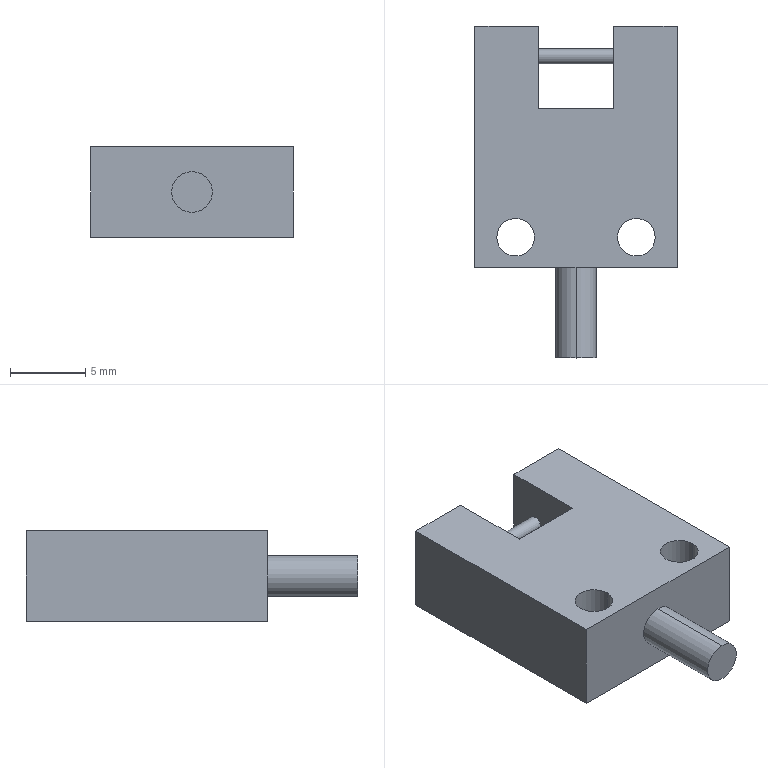Part | SolidWorks | features ICE 3, Extrusion 1, HoleWzd 1 | 1 solid | 19 faces | box 13.4 x 22 x 6 mm | volume 1101 mm3 | plane 11 | cylinder 8 | commonest cylinder face diameters 2.5 x4 1 x2 2.7 x2
STEP:
#1=CARTESIAN_POINT('',(-2.5,6.5,0.));
#2=VERTEX_POINT('',#1);
#3=CARTESIAN_POINT('',(-2.5,5.5,0.));
#4=VERTEX_POINT('',#3);
#5=CARTESIAN_POINT('',(-2.5,6.,0.));
#6=DIRECTION('',(1.,0.,0.));
#7=DIRECTION('',(0.,-1.,0.));
#8=AXIS2_PLACEMENT_3D('',#5,#6,#7);
#9=CIRCLE('',#8,0.5);
#10=EDGE_CURVE('',#2,#4,#9,.T.);
#11=ORIENTED_EDGE('',*,*,#10,.T.);
#12=CARTESIAN_POINT('',(2.5,5.5,0.));
#13=VERTEX_POINT('',#12);
#14=CARTESIAN_POINT('',(-3.914,5.5,0.));
#15=DIRECTION('',(1.,0.,0.));
#16=VECTOR('',#15,1000.);
#17=LINE('',#14,#16);
#18=EDGE_CURVE('',#4,#13,#17,.T.);
#19=ORIENTED_EDGE('',*,*,#18,.T.);
#20=CARTESIAN_POINT('',(2.5,6.5,0.));
#21=VERTEX_POINT('',#20);
#22=CARTESIAN_POINT('',(2.5,6.,0.));
#23=DIRECTION('',(-1.,0.,0.));
#24=DIRECTION('',(0.,1.,0.));
#25=AXIS2_PLACEMENT_3D('',#22,#23,#24);
#26=CIRCLE('',#25,0.5);
#27=EDGE_CURVE('',#13,#21,#26,.T.);
#28=ORIENTED_EDGE('',*,*,#27,.T.);
#29=CARTESIAN_POINT('',(-3.914,6.5,0.));
#30=DIRECTION('',(1.,0.,0.));
#31=VECTOR('',#30,1000.);
#32=LINE('',#29,#31);
#33=EDGE_CURVE('',#2,#21,#32,.T.);
#34=ORIENTED_EDGE('',*,*,#33,.F.);
#35=EDGE_LOOP('',(#11,#19,#28,#34));
#36=FACE_OUTER_BOUND('',#35,.T.);
#37=CARTESIAN_POINT('',(-3.914,6.,0.));
#38=DIRECTION('',(1.,0.,0.));
#39=DIRECTION('',(0.,1.,0.));
#40=AXIS2_PLACEMENT_3D('',#37,#38,#39);
#41=CYLINDRICAL_SURFACE('',#40,0.5);
#42=ADVANCED_FACE('',(#36),#41,.T.);
#43=CARTESIAN_POINT('',(-5.25,-6.,-3.));
#44=VERTEX_POINT('',#43);
#45=CARTESIAN_POINT('',(-2.75,-6.,-3.));
#46=VERTEX_POINT('',#45);
#47=CARTESIAN_POINT('',(-4.,-6.,-3.));
#48=DIRECTION('',(0.,0.,1.));
#49=DIRECTION('',(1.,0.,0.));
#50=AXIS2_PLACEMENT_3D('',#47,#48,#49);
#51=CIRCLE('',#50,1.25);
#52=EDGE_CURVE('',#44,#46,#51,.T.);
#53=ORIENTED_EDGE('',*,*,#52,.F.);
#54=CARTESIAN_POINT('',(-5.25,-6.,3.));
#55=VERTEX_POINT('',#54);
#56=CARTESIAN_POINT('',(-5.25,-6.,3.));
#57=DIRECTION('',(0.,0.,1.));
#58=VECTOR('',#57,1000.);
#59=LINE('',#56,#58);
#60=EDGE_CURVE('',#44,#55,#59,.T.);
#61=ORIENTED_EDGE('',*,*,#60,.T.);
#62=CARTESIAN_POINT('',(-2.75,-6.,3.));
#63=VERTEX_POINT('',#62);
#64=CARTESIAN_POINT('',(-4.,-6.,3.));
#65=DIRECTION('',(0.,0.,1.));
#66=DIRECTION('',(1.,0.,0.));
#67=AXIS2_PLACEMENT_3D('',#64,#65,#66);
#68=CIRCLE('',#67,1.25);
#69=EDGE_CURVE('',#55,#63,#68,.T.);
#70=ORIENTED_EDGE('',*,*,#69,.T.);
#71=CARTESIAN_POINT('',(-2.75,-6.,3.));
#72=DIRECTION('',(0.,0.,1.));
#73=VECTOR('',#72,1000.);
#74=LINE('',#71,#73);
#75=EDGE_CURVE('',#46,#63,#74,.T.);
#76=ORIENTED_EDGE('',*,*,#75,.F.);
#77=EDGE_LOOP('',(#53,#61,#70,#76));
#78=FACE_OUTER_BOUND('',#77,.T.);
#79=CARTESIAN_POINT('',(-4.,-6.,3.));
#80=DIRECTION('',(0.,0.,1.));
#81=DIRECTION('',(1.,0.,0.));
#82=AXIS2_PLACEMENT_3D('',#79,#80,#81);
#83=CYLINDRICAL_SURFACE('',#82,1.25);
#84=ADVANCED_FACE('',(#78),#83,.F.);
#85=CARTESIAN_POINT('',(2.75,-6.,-3.));
#86=VERTEX_POINT('',#85);
#87=CARTESIAN_POINT('',(5.25,-6.,-3.));
#88=VERTEX_POINT('',#87);
#89=CARTESIAN_POINT('',(4.,-6.,-3.));
#90=DIRECTION('',(0.,0.,1.));
#91=DIRECTION('',(1.,0.,0.));
#92=AXIS2_PLACEMENT_3D('',#89,#90,#91);
#93=CIRCLE('',#92,1.25);
#94=EDGE_CURVE('',#86,#88,#93,.T.);
#95=ORIENTED_EDGE('',*,*,#94,.F.);
#96=CARTESIAN_POINT('',(2.75,-6.,3.));
#97=VERTEX_POINT('',#96);
#98=CARTESIAN_POINT('',(2.75,-6.,3.));
#99=DIRECTION('',(0.,0.,1.));
#100=VECTOR('',#99,1000.);
#101=LINE('',#98,#100);
#102=EDGE_CURVE('',#86,#97,#101,.T.);
#103=ORIENTED_EDGE('',*,*,#102,.T.);
#104=CARTESIAN_POINT('',(5.25,-6.,3.));
#105=VERTEX_POINT('',#104);
#106=CARTESIAN_POINT('',(4.,-6.,3.));
#107=DIRECTION('',(0.,0.,1.));
#108=DIRECTION('',(1.,0.,0.));
#109=AXIS2_PLACEMENT_3D('',#106,#107,#108);
#110=CIRCLE('',#109,1.25);
#111=EDGE_CURVE('',#97,#105,#110,.T.);
#112=ORIENTED_EDGE('',*,*,#111,.T.);
#113=CARTESIAN_POINT('',(5.25,-6.,3.));
#114=DIRECTION('',(0.,0.,1.));
#115=VECTOR('',#114,1000.);
#116=LINE('',#113,#115);
#117=EDGE_CURVE('',#88,#105,#116,.T.);
#118=ORIENTED_EDGE('',*,*,#117,.F.);
#119=EDGE_LOOP('',(#95,#103,#112,#118));
#120=FACE_OUTER_BOUND('',#119,.T.);
#121=CARTESIAN_POINT('',(4.,-6.,3.));
#122=DIRECTION('',(0.,0.,1.));
#123=DIRECTION('',(1.,0.,0.));
#124=AXIS2_PLACEMENT_3D('',#121,#122,#123);
#125=CYLINDRICAL_SURFACE('',#124,1.25);
#126=ADVANCED_FACE('',(#120),#125,.F.);
#127=CARTESIAN_POINT('',(0.,-14.,-1.35));
#128=VERTEX_POINT('',#127);
#129=CARTESIAN_POINT('',(0.,-14.,1.35));
#130=VERTEX_POINT('',#129);
#131=CARTESIAN_POINT('',(0.,-14.,0.));
#132=DIRECTION('',(0.,-1.,0.));
#133=DIRECTION('',(0.,0.,-1.));
#134=AXIS2_PLACEMENT_3D('',#131,#132,#133);
#135=CIRCLE('',#134,1.35);
#136=EDGE_CURVE('',#128,#130,#135,.T.);
#137=ORIENTED_EDGE('',*,*,#136,.F.);
#138=CARTESIAN_POINT('',(0.,-8.,-1.35));
#139=VERTEX_POINT('',#138);
#140=CARTESIAN_POINT('',(0.,-14.,-1.35));
#141=DIRECTION('',(0.,1.,0.));
#142=VECTOR('',#141,1000.);
#143=LINE('',#140,#142);
#144=EDGE_CURVE('',#128,#139,#143,.T.);
#145=ORIENTED_EDGE('',*,*,#144,.T.);
#146=CARTESIAN_POINT('',(0.,-8.,1.35));
#147=VERTEX_POINT('',#146);
#148=CARTESIAN_POINT('',(0.,-8.,0.));
#149=DIRECTION('',(0.,-1.,0.));
#150=DIRECTION('',(0.,0.,1.));
#151=AXIS2_PLACEMENT_3D('',#148,#149,#150);
#152=CIRCLE('',#151,1.35);
#153=EDGE_CURVE('',#139,#147,#152,.T.);
#154=ORIENTED_EDGE('',*,*,#153,.T.);
#155=CARTESIAN_POINT('',(0.,-14.,1.35));
#156=DIRECTION('',(0.,1.,0.));
#157=VECTOR('',#156,1000.);
#158=LINE('',#155,#157);
#159=EDGE_CURVE('',#130,#147,#158,.T.);
#160=ORIENTED_EDGE('',*,*,#159,.F.);
#161=EDGE_LOOP('',(#137,#145,#154,#160));
#162=FACE_OUTER_BOUND('',#161,.T.);
#163=CARTESIAN_POINT('',(0.,-14.,0.));
#164=DIRECTION('',(0.,1.,0.));
#165=DIRECTION('',(0.,0.,1.));
#166=AXIS2_PLACEMENT_3D('',#163,#164,#165);
#167=CYLINDRICAL_SURFACE('',#166,1.35);
#168=ADVANCED_FACE('',(#162),#167,.T.);
#169=CARTESIAN_POINT('',(-2.5,8.,3.));
#170=VERTEX_POINT('',#169);
#171=CARTESIAN_POINT('',(-2.5,2.5,3.));
#172=VERTEX_POINT('',#171);
#173=CARTESIAN_POINT('',(-2.5,8.,3.));
#174=DIRECTION('',(0.,-1.,0.));
#175=VECTOR('',#174,1000.);
#176=LINE('',#173,#175);
#177=EDGE_CURVE('',#170,#172,#176,.T.);
#178=ORIENTED_EDGE('',*,*,#177,.T.);
#179=CARTESIAN_POINT('',(-2.5,2.5,-3.));
#180=VERTEX_POINT('',#179);
#181=CARTESIAN_POINT('',(-2.5,2.5,-3.));
#182=DIRECTION('',(0.,0.,1.));
#183=VECTOR('',#182,1000.);
#184=LINE('',#181,#183);
#185=EDGE_CURVE('',#180,#172,#184,.T.);
#186=ORIENTED_EDGE('',*,*,#185,.F.);
#187=CARTESIAN_POINT('',(-2.5,8.,-3.));
#188=VERTEX_POINT('',#187);
#189=CARTESIAN_POINT('',(-2.5,8.,-3.));
#190=DIRECTION('',(0.,-1.,0.));
#191=VECTOR('',#190,1000.);
#192=LINE('',#189,#191);
#193=EDGE_CURVE('',#188,#180,#192,.T.);
#194=ORIENTED_EDGE('',*,*,#193,.F.);
#195=CARTESIAN_POINT('',(-2.5,8.,-3.));
#196=DIRECTION('',(0.,0.,1.));
#197=VECTOR('',#196,1000.);
#198=LINE('',#195,#197);
#199=EDGE_CURVE('',#188,#170,#198,.T.);
#200=ORIENTED_EDGE('',*,*,#199,.T.);
#201=EDGE_LOOP('',(#178,#186,#194,#200));
#202=FACE_OUTER_BOUND('',#201,.T.);
#203=ORIENTED_EDGE('',*,*,#10,.F.);
#204=CARTESIAN_POINT('',(-2.5,6.,0.));
#205=DIRECTION('',(1.,0.,0.));
#206=DIRECTION('',(0.,-1.,0.));
#207=AXIS2_PLACEMENT_3D('',#204,#205,#206);
#208=CIRCLE('',#207,0.5);
#209=EDGE_CURVE('',#4,#2,#208,.T.);
#210=ORIENTED_EDGE('',*,*,#209,.F.);
#211=EDGE_LOOP('',(#203,#210));
#212=FACE_BOUND('',#211,.T.);
#213=CARTESIAN_POINT('',(-2.5,8.,-3.));
#214=DIRECTION('',(-1.,0.,0.));
#215=DIRECTION('',(0.,-1.,0.));
#216=AXIS2_PLACEMENT_3D('',#213,#214,#215);
#217=PLANE('',#216);
#218=ADVANCED_FACE('',(#202,#212),#217,.F.);
#219=CARTESIAN_POINT('',(2.5,2.5,3.));
#220=VERTEX_POINT('',#219);
#221=CARTESIAN_POINT('',(2.5,8.,3.));
#222=VERTEX_POINT('',#221);
#223=CARTESIAN_POINT('',(2.5,8.,3.));
#224=DIRECTION('',(0.,1.,0.));
#225=VECTOR('',#224,1000.);
#226=LINE('',#223,#225);
#227=EDGE_CURVE('',#220,#222,#226,.T.);
#228=ORIENTED_EDGE('',*,*,#227,.T.);
#229=CARTESIAN_POINT('',(2.5,8.,-3.));
#230=VERTEX_POINT('',#229);
#231=CARTESIAN_POINT('',(2.5,8.,-3.));
#232=DIRECTION('',(0.,0.,1.));
#233=VECTOR('',#232,1000.);
#234=LINE('',#231,#233);
#235=EDGE_CURVE('',#230,#222,#234,.T.);
#236=ORIENTED_EDGE('',*,*,#235,.F.);
#237=CARTESIAN_POINT('',(2.5,2.5,-3.));
#238=VERTEX_POINT('',#237);
#239=CARTESIAN_POINT('',(2.5,8.,-3.));
#240=DIRECTION('',(0.,1.,0.));
#241=VECTOR('',#240,1000.);
#242=LINE('',#239,#241);
#243=EDGE_CURVE('',#238,#230,#242,.T.);
#244=ORIENTED_EDGE('',*,*,#243,.F.);
#245=CARTESIAN_POINT('',(2.5,2.5,-3.));
#246=DIRECTION('',(0.,0.,1.));
#247=VECTOR('',#246,1000.);
#248=LINE('',#245,#247);
#249=EDGE_CURVE('',#238,#220,#248,.T.);
#250=ORIENTED_EDGE('',*,*,#249,.T.);
#251=EDGE_LOOP('',(#228,#236,#244,#250));
#252=FACE_OUTER_BOUND('',#251,.T.);
#253=CARTESIAN_POINT('',(2.5,6.,0.));
#254=DIRECTION('',(-1.,0.,0.));
#255=DIRECTION('',(0.,1.,0.));
#256=AXIS2_PLACEMENT_3D('',#253,#254,#255);
#257=CIRCLE('',#256,0.5);
#258=EDGE_CURVE('',#21,#13,#257,.T.);
#259=ORIENTED_EDGE('',*,*,#258,.F.);
#260=ORIENTED_EDGE('',*,*,#27,.F.);
#261=EDGE_LOOP('',(#259,#260));
#262=FACE_BOUND('',#261,.T.);
#263=CARTESIAN_POINT('',(2.5,8.,-3.));
#264=DIRECTION('',(1.,0.,0.));
#265=DIRECTION('',(0.,1.,0.));
#266=AXIS2_PLACEMENT_3D('',#263,#264,#265);
#267=PLANE('',#266);
#268=ADVANCED_FACE('',(#252,#262),#267,.F.);
#269=CARTESIAN_POINT('',(-6.7,-8.,-3.));
#270=VERTEX_POINT('',#269);
#271=CARTESIAN_POINT('',(6.7,-8.,-3.));
#272=VERTEX_POINT('',#271);
#273=CARTESIAN_POINT('',(-6.7,-8.,-3.));
#274=DIRECTION('',(1.,0.,0.));
#275=VECTOR('',#274,1000.);
#276=LINE('',#273,#275);
#277=EDGE_CURVE('',#270,#272,#276,.T.);
#278=ORIENTED_EDGE('',*,*,#277,.T.);
#279=CARTESIAN_POINT('',(6.7,-8.,3.));
#280=VERTEX_POINT('',#279);
#281=CARTESIAN_POINT('',(6.7,-8.,3.));
#282=DIRECTION('',(0.,0.,-1.));
#283=VECTOR('',#282,1000.);
#284=LINE('',#281,#283);
#285=EDGE_CURVE('',#280,#272,#284,.T.);
#286=ORIENTED_EDGE('',*,*,#285,.F.);
#287=CARTESIAN_POINT('',(-6.7,-8.,3.));
#288=VERTEX_POINT('',#287);
#289=CARTESIAN_POINT('',(-6.7,-8.,3.));
#290=DIRECTION('',(1.,0.,0.));
#291=VECTOR('',#290,1000.);
#292=LINE('',#289,#291);
#293=EDGE_CURVE('',#288,#280,#292,.T.);
#294=ORIENTED_EDGE('',*,*,#293,.F.);
#295=CARTESIAN_POINT('',(-6.7,-8.,3.));
#296=DIRECTION('',(0.,0.,-1.));
#297=VECTOR('',#296,1000.);
#298=LINE('',#295,#297);
#299=EDGE_CURVE('',#288,#270,#298,.T.);
#300=ORIENTED_EDGE('',*,*,#299,.T.);
#301=EDGE_LOOP('',(#278,#286,#294,#300));
#302=FACE_OUTER_BOUND('',#301,.T.);
#303=CARTESIAN_POINT('',(0.,-8.,0.));
#304=DIRECTION('',(0.,-1.,0.));
#305=DIRECTION('',(0.,0.,1.));
#306=AXIS2_PLACEMENT_3D('',#303,#304,#305);
#307=CIRCLE('',#306,1.35);
#308=EDGE_CURVE('',#147,#139,#307,.T.);
#309=ORIENTED_EDGE('',*,*,#308,.F.);
#310=ORIENTED_EDGE('',*,*,#153,.F.);
#311=EDGE_LOOP('',(#309,#310));
#312=FACE_BOUND('',#311,.T.);
#313=CARTESIAN_POINT('',(-6.7,-8.,3.));
#314=DIRECTION('',(0.,1.,0.));
#315=DIRECTION('',(0.,0.,1.));
#316=AXIS2_PLACEMENT_3D('',#313,#314,#315);
#317=PLANE('',#316);
#318=ADVANCED_FACE('',(#302,#312),#317,.F.);
#319=CARTESIAN_POINT('',(-6.7,8.,3.));
#320=VERTEX_POINT('',#319);
#321=CARTESIAN_POINT('',(-6.7,8.,3.));
#322=DIRECTION('',(-1.,0.,0.));
#323=VECTOR('',#322,1000.);
#324=LINE('',#321,#323);
#325=EDGE_CURVE('',#170,#320,#324,.T.);
#326=ORIENTED_EDGE('',*,*,#325,.F.);
#327=ORIENTED_EDGE('',*,*,#199,.F.);
#328=CARTESIAN_POINT('',(-6.7,8.,-3.));
#329=VERTEX_POINT('',#328);
#330=CARTESIAN_POINT('',(-6.7,8.,-3.));
#331=DIRECTION('',(-1.,0.,0.));
#332=VECTOR('',#331,1000.);
#333=LINE('',#330,#332);
#334=EDGE_CURVE('',#188,#329,#333,.T.);
#335=ORIENTED_EDGE('',*,*,#334,.T.);
#336=CARTESIAN_POINT('',(-6.7,8.,3.));
#337=DIRECTION('',(0.,0.,-1.));
#338=VECTOR('',#337,1000.);
#339=LINE('',#336,#338);
#340=EDGE_CURVE('',#320,#329,#339,.T.);
#341=ORIENTED_EDGE('',*,*,#340,.F.);
#342=EDGE_LOOP('',(#326,#327,#335,#341));
#343=FACE_OUTER_BOUND('',#342,.T.);
#344=CARTESIAN_POINT('',(-6.7,8.,3.));
#345=DIRECTION('',(0.,-1.,0.));
#346=DIRECTION('',(0.,0.,-1.));
#347=AXIS2_PLACEMENT_3D('',#344,#345,#346);
#348=PLANE('',#347);
#349=ADVANCED_FACE('',(#343),#348,.F.);
#350=CARTESIAN_POINT('',(6.7,8.,-3.));
#351=VERTEX_POINT('',#350);
#352=CARTESIAN_POINT('',(6.7,8.,-3.));
#353=DIRECTION('',(0.,1.,0.));
#354=VECTOR('',#353,1000.);
#355=LINE('',#352,#354);
#356=EDGE_CURVE('',#272,#351,#355,.T.);
#357=ORIENTED_EDGE('',*,*,#356,.T.);
#358=CARTESIAN_POINT('',(6.7,8.,3.));
#359=VERTEX_POINT('',#358);
#360=CARTESIAN_POINT('',(6.7,8.,3.));
#361=DIRECTION('',(0.,0.,-1.));
#362=VECTOR('',#361,1000.);
#363=LINE('',#360,#362);
#364=EDGE_CURVE('',#359,#351,#363,.T.);
#365=ORIENTED_EDGE('',*,*,#364,.F.);
#366=CARTESIAN_POINT('',(6.7,8.,3.));
#367=DIRECTION('',(0.,1.,0.));
#368=VECTOR('',#367,1000.);
#369=LINE('',#366,#368);
#370=EDGE_CURVE('',#280,#359,#369,.T.);
#371=ORIENTED_EDGE('',*,*,#370,.F.);
#372=ORIENTED_EDGE('',*,*,#285,.T.);
#373=EDGE_LOOP('',(#357,#365,#371,#372));
#374=FACE_OUTER_BOUND('',#373,.T.);
#375=CARTESIAN_POINT('',(6.7,8.,3.));
#376=DIRECTION('',(-1.,0.,0.));
#377=DIRECTION('',(0.,-1.,0.));
#378=AXIS2_PLACEMENT_3D('',#375,#376,#377);
#379=PLANE('',#378);
#380=ADVANCED_FACE('',(#374),#379,.F.);
#381=CARTESIAN_POINT('',(-6.7,8.,-3.));
#382=DIRECTION('',(-1.,0.,0.));
#383=VECTOR('',#382,1000.);
#384=LINE('',#381,#383);
#385=EDGE_CURVE('',#351,#230,#384,.T.);
#386=ORIENTED_EDGE('',*,*,#385,.T.);
#387=ORIENTED_EDGE('',*,*,#235,.T.);
#388=CARTESIAN_POINT('',(-6.7,8.,3.));
#389=DIRECTION('',(-1.,0.,0.));
#390=VECTOR('',#389,1000.);
#391=LINE('',#388,#390);
#392=EDGE_CURVE('',#359,#222,#391,.T.);
#393=ORIENTED_EDGE('',*,*,#392,.F.);
#394=ORIENTED_EDGE('',*,*,#364,.T.);
#395=EDGE_LOOP('',(#386,#387,#393,#394));
#396=FACE_OUTER_BOUND('',#395,.T.);
#397=CARTESIAN_POINT('',(-6.7,8.,3.));
#398=DIRECTION('',(0.,-1.,0.));
#399=DIRECTION('',(0.,0.,-1.));
#400=AXIS2_PLACEMENT_3D('',#397,#398,#399);
#401=PLANE('',#400);
#402=ADVANCED_FACE('',(#396),#401,.F.);
#403=CARTESIAN_POINT('',(-6.7,8.,-3.));
#404=DIRECTION('',(0.,-1.,0.));
#405=VECTOR('',#404,1000.);
#406=LINE('',#403,#405);
#407=EDGE_CURVE('',#329,#270,#406,.T.);
#408=ORIENTED_EDGE('',*,*,#407,.T.);
#409=ORIENTED_EDGE('',*,*,#299,.F.);
#410=CARTESIAN_POINT('',(-6.7,8.,3.));
#411=DIRECTION('',(0.,-1.,0.));
#412=VECTOR('',#411,1000.);
#413=LINE('',#410,#412);
#414=EDGE_CURVE('',#320,#288,#413,.T.);
#415=ORIENTED_EDGE('',*,*,#414,.F.);
#416=ORIENTED_EDGE('',*,*,#340,.T.);
#417=EDGE_LOOP('',(#408,#409,#415,#416));
#418=FACE_OUTER_BOUND('',#417,.T.);
#419=CARTESIAN_POINT('',(-6.7,8.,3.));
#420=DIRECTION('',(1.,0.,0.));
#421=DIRECTION('',(0.,1.,0.));
#422=AXIS2_PLACEMENT_3D('',#419,#420,#421);
#423=PLANE('',#422);
#424=ADVANCED_FACE('',(#418),#423,.F.);
#425=CARTESIAN_POINT('',(-4.,-6.,3.));
#426=DIRECTION('',(0.,0.,1.));
#427=DIRECTION('',(1.,0.,0.));
#428=AXIS2_PLACEMENT_3D('',#425,#426,#427);
#429=CIRCLE('',#428,1.25);
#430=EDGE_CURVE('',#63,#55,#429,.T.);
#431=ORIENTED_EDGE('',*,*,#430,.F.);
#432=ORIENTED_EDGE('',*,*,#69,.F.);
#433=EDGE_LOOP('',(#431,#432));
#434=FACE_BOUND('',#433,.T.);
#435=CARTESIAN_POINT('',(4.,-6.,3.));
#436=DIRECTION('',(0.,0.,1.));
#437=DIRECTION('',(1.,0.,0.));
#438=AXIS2_PLACEMENT_3D('',#435,#436,#437);
#439=CIRCLE('',#438,1.25);
#440=EDGE_CURVE('',#105,#97,#439,.T.);
#441=ORIENTED_EDGE('',*,*,#440,.F.);
#442=ORIENTED_EDGE('',*,*,#111,.F.);
#443=EDGE_LOOP('',(#441,#442));
#444=FACE_BOUND('',#443,.T.);
#445=ORIENTED_EDGE('',*,*,#177,.F.);
#446=ORIENTED_EDGE('',*,*,#325,.T.);
#447=ORIENTED_EDGE('',*,*,#414,.T.);
#448=ORIENTED_EDGE('',*,*,#293,.T.);
#449=ORIENTED_EDGE('',*,*,#370,.T.);
#450=ORIENTED_EDGE('',*,*,#392,.T.);
#451=ORIENTED_EDGE('',*,*,#227,.F.);
#452=CARTESIAN_POINT('',(-2.5,2.5,3.));
#453=DIRECTION('',(1.,0.,0.));
#454=VECTOR('',#453,1000.);
#455=LINE('',#452,#454);
#456=EDGE_CURVE('',#172,#220,#455,.T.);
#457=ORIENTED_EDGE('',*,*,#456,.F.);
#458=EDGE_LOOP('',(#445,#446,#447,#448,#449,#450,#451,#457));
#459=FACE_OUTER_BOUND('',#458,.T.);
#460=CARTESIAN_POINT('',(0.,0.,3.));
#461=DIRECTION('',(0.,0.,1.));
#462=DIRECTION('',(1.,0.,0.));
#463=AXIS2_PLACEMENT_3D('',#460,#461,#462);
#464=PLANE('',#463);
#465=ADVANCED_FACE('',(#434,#444,#459),#464,.T.);
#466=CARTESIAN_POINT('',(-4.,-6.,-3.));
#467=DIRECTION('',(0.,0.,1.));
#468=DIRECTION('',(1.,0.,0.));
#469=AXIS2_PLACEMENT_3D('',#466,#467,#468);
#470=CIRCLE('',#469,1.25);
#471=EDGE_CURVE('',#46,#44,#470,.T.);
#472=ORIENTED_EDGE('',*,*,#471,.T.);
#473=ORIENTED_EDGE('',*,*,#52,.T.);
#474=EDGE_LOOP('',(#472,#473));
#475=FACE_BOUND('',#474,.T.);
#476=CARTESIAN_POINT('',(4.,-6.,-3.));
#477=DIRECTION('',(0.,0.,1.));
#478=DIRECTION('',(1.,0.,0.));
#479=AXIS2_PLACEMENT_3D('',#476,#477,#478);
#480=CIRCLE('',#479,1.25);
#481=EDGE_CURVE('',#88,#86,#480,.T.);
#482=ORIENTED_EDGE('',*,*,#481,.T.);
#483=ORIENTED_EDGE('',*,*,#94,.T.);
#484=EDGE_LOOP('',(#482,#483));
#485=FACE_BOUND('',#484,.T.);
#486=ORIENTED_EDGE('',*,*,#334,.F.);
#487=ORIENTED_EDGE('',*,*,#193,.T.);
#488=CARTESIAN_POINT('',(-2.5,2.5,-3.));
#489=DIRECTION('',(1.,0.,0.));
#490=VECTOR('',#489,1000.);
#491=LINE('',#488,#490);
#492=EDGE_CURVE('',#180,#238,#491,.T.);
#493=ORIENTED_EDGE('',*,*,#492,.T.);
#494=ORIENTED_EDGE('',*,*,#243,.T.);
#495=ORIENTED_EDGE('',*,*,#385,.F.);
#496=ORIENTED_EDGE('',*,*,#356,.F.);
#497=ORIENTED_EDGE('',*,*,#277,.F.);
#498=ORIENTED_EDGE('',*,*,#407,.F.);
#499=EDGE_LOOP('',(#486,#487,#493,#494,#495,#496,#497,#498));
#500=FACE_OUTER_BOUND('',#499,.T.);
#501=CARTESIAN_POINT('',(0.,0.,-3.));
#502=DIRECTION('',(0.,0.,1.));
#503=DIRECTION('',(1.,0.,0.));
#504=AXIS2_PLACEMENT_3D('',#501,#502,#503);
#505=PLANE('',#504);
#506=ADVANCED_FACE('',(#475,#485,#500),#505,.F.);
#507=ORIENTED_EDGE('',*,*,#456,.T.);
#508=ORIENTED_EDGE('',*,*,#249,.F.);
#509=ORIENTED_EDGE('',*,*,#492,.F.);
#510=ORIENTED_EDGE('',*,*,#185,.T.);
#511=EDGE_LOOP('',(#507,#508,#509,#510));
#512=FACE_OUTER_BOUND('',#511,.T.);
#513=CARTESIAN_POINT('',(-2.5,2.5,-3.));
#514=DIRECTION('',(0.,-1.,0.));
#515=DIRECTION('',(0.,0.,-1.));
#516=AXIS2_PLACEMENT_3D('',#513,#514,#515);
#517=PLANE('',#516);
#518=ADVANCED_FACE('',(#512),#517,.F.);
#519=ORIENTED_EDGE('',*,*,#144,.F.);
#520=CARTESIAN_POINT('',(0.,-14.,0.));
#521=DIRECTION('',(0.,-1.,0.));
#522=DIRECTION('',(0.,0.,-1.));
#523=AXIS2_PLACEMENT_3D('',#520,#521,#522);
#524=CIRCLE('',#523,1.35);
#525=EDGE_CURVE('',#130,#128,#524,.T.);
#526=ORIENTED_EDGE('',*,*,#525,.F.);
#527=ORIENTED_EDGE('',*,*,#159,.T.);
#528=ORIENTED_EDGE('',*,*,#308,.T.);
#529=EDGE_LOOP('',(#519,#526,#527,#528));
#530=FACE_OUTER_BOUND('',#529,.T.);
#531=CARTESIAN_POINT('',(0.,-14.,0.));
#532=DIRECTION('',(0.,1.,0.));
#533=DIRECTION('',(0.,0.,1.));
#534=AXIS2_PLACEMENT_3D('',#531,#532,#533);
#535=CYLINDRICAL_SURFACE('',#534,1.35);
#536=ADVANCED_FACE('',(#530),#535,.T.);
#537=ORIENTED_EDGE('',*,*,#525,.T.);
#538=ORIENTED_EDGE('',*,*,#136,.T.);
#539=EDGE_LOOP('',(#537,#538));
#540=FACE_OUTER_BOUND('',#539,.T.);
#541=CARTESIAN_POINT('',(0.,-14.,0.));
#542=DIRECTION('',(0.,-1.,0.));
#543=DIRECTION('',(0.,0.,-1.));
#544=AXIS2_PLACEMENT_3D('',#541,#542,#543);
#545=PLANE('',#544);
#546=ADVANCED_FACE('',(#540),#545,.T.);
#547=ORIENTED_EDGE('',*,*,#102,.F.);
#548=ORIENTED_EDGE('',*,*,#481,.F.);
#549=ORIENTED_EDGE('',*,*,#117,.T.);
#550=ORIENTED_EDGE('',*,*,#440,.T.);
#551=EDGE_LOOP('',(#547,#548,#549,#550));
#552=FACE_OUTER_BOUND('',#551,.T.);
#553=CARTESIAN_POINT('',(4.,-6.,3.));
#554=DIRECTION('',(0.,0.,1.));
#555=DIRECTION('',(1.,0.,0.));
#556=AXIS2_PLACEMENT_3D('',#553,#554,#555);
#557=CYLINDRICAL_SURFACE('',#556,1.25);
#558=ADVANCED_FACE('',(#552),#557,.F.);
#559=ORIENTED_EDGE('',*,*,#60,.F.);
#560=ORIENTED_EDGE('',*,*,#471,.F.);
#561=ORIENTED_EDGE('',*,*,#75,.T.);
#562=ORIENTED_EDGE('',*,*,#430,.T.);
#563=EDGE_LOOP('',(#559,#560,#561,#562));
#564=FACE_OUTER_BOUND('',#563,.T.);
#565=CARTESIAN_POINT('',(-4.,-6.,3.));
#566=DIRECTION('',(0.,0.,1.));
#567=DIRECTION('',(1.,0.,0.));
#568=AXIS2_PLACEMENT_3D('',#565,#566,#567);
#569=CYLINDRICAL_SURFACE('',#568,1.25);
#570=ADVANCED_FACE('',(#564),#569,.F.);
#571=ORIENTED_EDGE('',*,*,#18,.F.);
#572=ORIENTED_EDGE('',*,*,#209,.T.);
#573=ORIENTED_EDGE('',*,*,#33,.T.);
#574=ORIENTED_EDGE('',*,*,#258,.T.);
#575=EDGE_LOOP('',(#571,#572,#573,#574));
#576=FACE_OUTER_BOUND('',#575,.T.);
#577=CARTESIAN_POINT('',(-3.914,6.,0.));
#578=DIRECTION('',(1.,0.,0.));
#579=DIRECTION('',(0.,1.,0.));
#580=AXIS2_PLACEMENT_3D('',#577,#578,#579);
#581=CYLINDRICAL_SURFACE('',#580,0.5);
#582=ADVANCED_FACE('',(#576),#581,.T.);
#583=CLOSED_SHELL('',(#42,#84,#126,#168,#218,#268,#318,#349,#380,#402,#424,#465,#506,#518,#536,#546,#558,#570,#582));
#584=MANIFOLD_SOLID_BREP('',#583);
#585=CARTESIAN_POINT('',(0.,0.,0.));
#586=DIRECTION('',(0.,0.,1.));
#587=DIRECTION('',(1.,0.,0.));
#588=AXIS2_PLACEMENT_3D('',#585,#586,#587);
#589=(LENGTH_UNIT()NAMED_UNIT(*)SI_UNIT(.MILLI.,.METRE.));
#590=UNCERTAINTY_MEASURE_WITH_UNIT(LENGTH_MEASURE(0.00001),#589,'','');
#591=(NAMED_UNIT(*)PLANE_ANGLE_UNIT()SI_UNIT($,.RADIAN.));
#592=(NAMED_UNIT(*)SI_UNIT($,.STERADIAN.)SOLID_ANGLE_UNIT());
#593=(GEOMETRIC_REPRESENTATION_CONTEXT(3)GLOBAL_UNCERTAINTY_ASSIGNED_CONTEXT((#590))GLOBAL_UNIT_ASSIGNED_CONTEXT((#589,#591,#592))REPRESENTATION_CONTEXT('',''));
#594=ADVANCED_BREP_SHAPE_REPRESENTATION('',(#584,#588),#593);